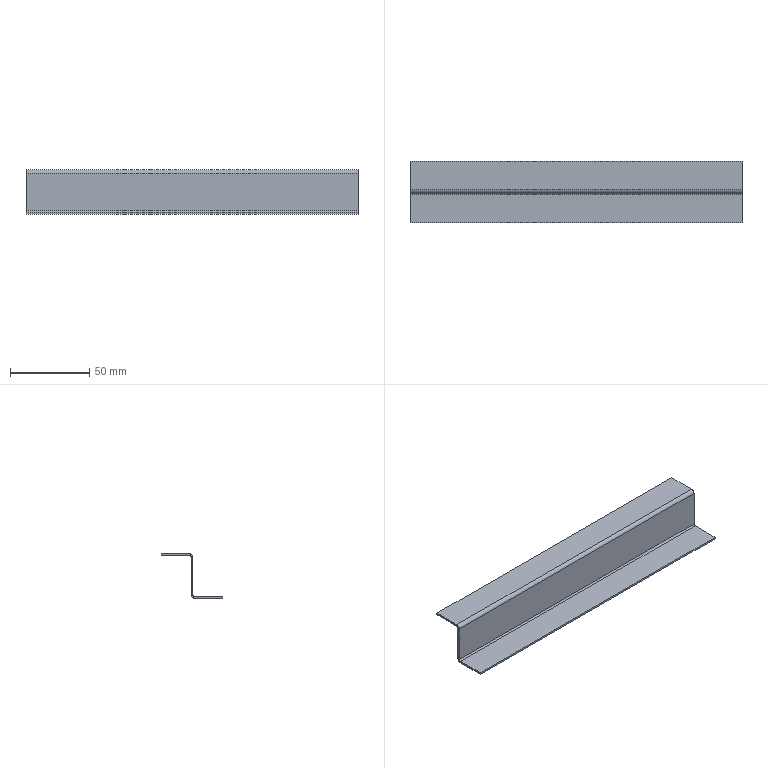Part | SolidWorks | features EdgeFlange 2, FlatPattern 1, HoleWzd 1, SMBaseFlange 1, SheetMetal 1 | 1 solid | 22 faces | box 210 x 38.8 x 28 mm | volume 16185 mm3 | plane 18 | cylinder 4 | commonest cylinder face diameters 2 x2 4.4 x2
STEP:
#1=CARTESIAN_POINT('',(105.,10.,24.6));
#2=VERTEX_POINT('',#1);
#3=CARTESIAN_POINT('',(105.,8.8,24.6));
#4=VERTEX_POINT('',#3);
#5=CARTESIAN_POINT('',(105.,10.,24.6));
#6=DIRECTION('',(0.,-1.,0.));
#7=VECTOR('',#6,1000.);
#8=LINE('',#5,#7);
#9=EDGE_CURVE('',#2,#4,#8,.T.);
#10=ORIENTED_EDGE('',*,*,#9,.T.);
#11=CARTESIAN_POINT('',(105.,8.8,1.));
#12=VERTEX_POINT('',#11);
#13=CARTESIAN_POINT('',(105.,8.8,0.));
#14=DIRECTION('',(0.,0.,-1.));
#15=VECTOR('',#14,1000.);
#16=LINE('',#13,#15);
#17=EDGE_CURVE('',#4,#12,#16,.T.);
#18=ORIENTED_EDGE('',*,*,#17,.T.);
#19=CARTESIAN_POINT('',(105.,10.,1.));
#20=VERTEX_POINT('',#19);
#21=CARTESIAN_POINT('',(105.,10.,1.));
#22=DIRECTION('',(0.,1.,0.));
#23=VECTOR('',#22,1000.);
#24=LINE('',#21,#23);
#25=EDGE_CURVE('',#12,#20,#24,.T.);
#26=ORIENTED_EDGE('',*,*,#25,.T.);
#27=CARTESIAN_POINT('',(105.,10.,0.));
#28=DIRECTION('',(0.,0.,-1.));
#29=VECTOR('',#28,1000.);
#30=LINE('',#27,#29);
#31=EDGE_CURVE('',#2,#20,#30,.T.);
#32=ORIENTED_EDGE('',*,*,#31,.F.);
#33=EDGE_LOOP('',(#10,#18,#26,#32));
#34=FACE_OUTER_BOUND('',#33,.T.);
#35=CARTESIAN_POINT('',(105.,10.,0.));
#36=DIRECTION('',(-1.,0.,0.));
#37=DIRECTION('',(0.,0.,1.));
#38=AXIS2_PLACEMENT_3D('',#35,#36,#37);
#39=PLANE('',#38);
#40=ADVANCED_FACE('',(#34),#39,.F.);
#41=CARTESIAN_POINT('',(-105.,10.,24.6));
#42=VERTEX_POINT('',#41);
#43=CARTESIAN_POINT('',(-105.,8.8,24.6));
#44=VERTEX_POINT('',#43);
#45=CARTESIAN_POINT('',(-105.,10.,24.6));
#46=DIRECTION('',(0.,-1.,0.));
#47=VECTOR('',#46,1000.);
#48=LINE('',#45,#47);
#49=EDGE_CURVE('',#42,#44,#48,.T.);
#50=ORIENTED_EDGE('',*,*,#49,.F.);
#51=CARTESIAN_POINT('',(-105.,10.,1.));
#52=VERTEX_POINT('',#51);
#53=CARTESIAN_POINT('',(-105.,10.,0.));
#54=DIRECTION('',(0.,0.,1.));
#55=VECTOR('',#54,1000.);
#56=LINE('',#53,#55);
#57=EDGE_CURVE('',#52,#42,#56,.T.);
#58=ORIENTED_EDGE('',*,*,#57,.F.);
#59=CARTESIAN_POINT('',(-105.,8.8,1.));
#60=VERTEX_POINT('',#59);
#61=CARTESIAN_POINT('',(-105.,8.8,1.));
#62=DIRECTION('',(0.,1.,0.));
#63=VECTOR('',#62,1000.);
#64=LINE('',#61,#63);
#65=EDGE_CURVE('',#60,#52,#64,.T.);
#66=ORIENTED_EDGE('',*,*,#65,.F.);
#67=CARTESIAN_POINT('',(-105.,8.8,26.8));
#68=DIRECTION('',(0.,0.,1.));
#69=VECTOR('',#68,1000.);
#70=LINE('',#67,#69);
#71=EDGE_CURVE('',#60,#44,#70,.T.);
#72=ORIENTED_EDGE('',*,*,#71,.T.);
#73=EDGE_LOOP('',(#50,#58,#66,#72));
#74=FACE_OUTER_BOUND('',#73,.T.);
#75=CARTESIAN_POINT('',(-105.,10.,26.8));
#76=DIRECTION('',(1.,0.,0.));
#77=DIRECTION('',(0.,0.,-1.));
#78=AXIS2_PLACEMENT_3D('',#75,#76,#77);
#79=PLANE('',#78);
#80=ADVANCED_FACE('',(#74),#79,.F.);
#81=CARTESIAN_POINT('',(105.,10.,24.6));
#82=DIRECTION('',(-1.,0.,0.));
#83=VECTOR('',#82,1000.);
#84=LINE('',#81,#83);
#85=EDGE_CURVE('',#2,#42,#84,.T.);
#86=ORIENTED_EDGE('',*,*,#85,.F.);
#87=ORIENTED_EDGE('',*,*,#31,.T.);
#88=CARTESIAN_POINT('',(105.,10.,1.));
#89=DIRECTION('',(1.,0.,0.));
#90=VECTOR('',#89,1000.);
#91=LINE('',#88,#90);
#92=EDGE_CURVE('',#52,#20,#91,.T.);
#93=ORIENTED_EDGE('',*,*,#92,.F.);
#94=ORIENTED_EDGE('',*,*,#57,.T.);
#95=EDGE_LOOP('',(#86,#87,#93,#94));
#96=FACE_OUTER_BOUND('',#95,.T.);
#97=CARTESIAN_POINT('',(0.,10.,0.));
#98=DIRECTION('',(0.,-1.,0.));
#99=DIRECTION('',(0.,0.,-1.));
#100=AXIS2_PLACEMENT_3D('',#97,#98,#99);
#101=PLANE('',#100);
#102=ADVANCED_FACE('',(#96),#101,.F.);
#103=ORIENTED_EDGE('',*,*,#17,.F.);
#104=CARTESIAN_POINT('',(105.,8.8,24.6));
#105=DIRECTION('',(-1.,0.,0.));
#106=VECTOR('',#105,1000.);
#107=LINE('',#104,#106);
#108=EDGE_CURVE('',#4,#44,#107,.T.);
#109=ORIENTED_EDGE('',*,*,#108,.T.);
#110=ORIENTED_EDGE('',*,*,#71,.F.);
#111=CARTESIAN_POINT('',(105.,8.8,1.));
#112=DIRECTION('',(-1.,0.,0.));
#113=VECTOR('',#112,1000.);
#114=LINE('',#111,#113);
#115=EDGE_CURVE('',#12,#60,#114,.T.);
#116=ORIENTED_EDGE('',*,*,#115,.F.);
#117=EDGE_LOOP('',(#103,#109,#110,#116));
#118=FACE_OUTER_BOUND('',#117,.T.);
#119=CARTESIAN_POINT('',(0.,8.8,0.));
#120=DIRECTION('',(0.,-1.,0.));
#121=DIRECTION('',(0.,0.,-1.));
#122=AXIS2_PLACEMENT_3D('',#119,#120,#121);
#123=PLANE('',#122);
#124=ADVANCED_FACE('',(#118),#123,.T.);
#125=CARTESIAN_POINT('',(-105.,7.8,0.));
#126=VERTEX_POINT('',#125);
#127=CARTESIAN_POINT('',(-105.,-10.,0.));
#128=VERTEX_POINT('',#127);
#129=CARTESIAN_POINT('',(-105.,10.,0.));
#130=DIRECTION('',(0.,-1.,0.));
#131=VECTOR('',#130,1000.);
#132=LINE('',#129,#131);
#133=EDGE_CURVE('',#126,#128,#132,.T.);
#134=ORIENTED_EDGE('',*,*,#133,.F.);
#135=CARTESIAN_POINT('',(-105.,7.8,-1.2));
#136=VERTEX_POINT('',#135);
#137=CARTESIAN_POINT('',(-105.,7.8,0.));
#138=DIRECTION('',(0.,0.,-1.));
#139=VECTOR('',#138,1000.);
#140=LINE('',#137,#139);
#141=EDGE_CURVE('',#126,#136,#140,.T.);
#142=ORIENTED_EDGE('',*,*,#141,.T.);
#143=CARTESIAN_POINT('',(-105.,-10.,-1.2));
#144=VERTEX_POINT('',#143);
#145=CARTESIAN_POINT('',(-105.,10.,-1.2));
#146=DIRECTION('',(0.,-1.,0.));
#147=VECTOR('',#146,1000.);
#148=LINE('',#145,#147);
#149=EDGE_CURVE('',#136,#144,#148,.T.);
#150=ORIENTED_EDGE('',*,*,#149,.T.);
#151=CARTESIAN_POINT('',(-105.,-10.,-1.2));
#152=DIRECTION('',(0.,0.,1.));
#153=VECTOR('',#152,1000.);
#154=LINE('',#151,#153);
#155=EDGE_CURVE('',#144,#128,#154,.T.);
#156=ORIENTED_EDGE('',*,*,#155,.T.);
#157=EDGE_LOOP('',(#134,#142,#150,#156));
#158=FACE_OUTER_BOUND('',#157,.T.);
#159=CARTESIAN_POINT('',(-105.,10.,-1.2));
#160=DIRECTION('',(-1.,0.,0.));
#161=DIRECTION('',(0.,0.,1.));
#162=AXIS2_PLACEMENT_3D('',#159,#160,#161);
#163=PLANE('',#162);
#164=ADVANCED_FACE('',(#158),#163,.T.);
#165=CARTESIAN_POINT('',(105.,7.8,-1.2));
#166=VERTEX_POINT('',#165);
#167=CARTESIAN_POINT('',(-105.,7.8,-1.2));
#168=DIRECTION('',(1.,0.,0.));
#169=VECTOR('',#168,1000.);
#170=LINE('',#167,#169);
#171=EDGE_CURVE('',#136,#166,#170,.T.);
#172=ORIENTED_EDGE('',*,*,#171,.T.);
#173=CARTESIAN_POINT('',(105.,-10.,-1.2));
#174=VERTEX_POINT('',#173);
#175=CARTESIAN_POINT('',(105.,10.,-1.2));
#176=DIRECTION('',(0.,1.,0.));
#177=VECTOR('',#176,1000.);
#178=LINE('',#175,#177);
#179=EDGE_CURVE('',#174,#166,#178,.T.);
#180=ORIENTED_EDGE('',*,*,#179,.F.);
#181=CARTESIAN_POINT('',(-105.,-10.,-1.2));
#182=DIRECTION('',(1.,0.,0.));
#183=VECTOR('',#182,1000.);
#184=LINE('',#181,#183);
#185=EDGE_CURVE('',#144,#174,#184,.T.);
#186=ORIENTED_EDGE('',*,*,#185,.F.);
#187=ORIENTED_EDGE('',*,*,#149,.F.);
#188=EDGE_LOOP('',(#172,#180,#186,#187));
#189=FACE_OUTER_BOUND('',#188,.T.);
#190=CARTESIAN_POINT('',(0.,0.,-1.2));
#191=DIRECTION('',(0.,0.,1.));
#192=DIRECTION('',(1.,0.,0.));
#193=AXIS2_PLACEMENT_3D('',#190,#191,#192);
#194=PLANE('',#193);
#195=ADVANCED_FACE('',(#189),#194,.F.);
#196=CARTESIAN_POINT('',(105.,-10.,0.));
#197=VERTEX_POINT('',#196);
#198=CARTESIAN_POINT('',(105.,7.8,0.));
#199=VERTEX_POINT('',#198);
#200=CARTESIAN_POINT('',(105.,10.,0.));
#201=DIRECTION('',(0.,1.,0.));
#202=VECTOR('',#201,1000.);
#203=LINE('',#200,#202);
#204=EDGE_CURVE('',#197,#199,#203,.T.);
#205=ORIENTED_EDGE('',*,*,#204,.T.);
#206=CARTESIAN_POINT('',(-105.,7.8,0.));
#207=DIRECTION('',(1.,0.,0.));
#208=VECTOR('',#207,1000.);
#209=LINE('',#206,#208);
#210=EDGE_CURVE('',#126,#199,#209,.T.);
#211=ORIENTED_EDGE('',*,*,#210,.F.);
#212=ORIENTED_EDGE('',*,*,#133,.T.);
#213=CARTESIAN_POINT('',(-105.,-10.,0.));
#214=DIRECTION('',(1.,0.,0.));
#215=VECTOR('',#214,1000.);
#216=LINE('',#213,#215);
#217=EDGE_CURVE('',#128,#197,#216,.T.);
#218=ORIENTED_EDGE('',*,*,#217,.T.);
#219=EDGE_LOOP('',(#205,#211,#212,#218));
#220=FACE_OUTER_BOUND('',#219,.T.);
#221=CARTESIAN_POINT('',(0.,0.,0.));
#222=DIRECTION('',(0.,0.,1.));
#223=DIRECTION('',(1.,0.,0.));
#224=AXIS2_PLACEMENT_3D('',#221,#222,#223);
#225=PLANE('',#224);
#226=ADVANCED_FACE('',(#220),#225,.T.);
#227=CARTESIAN_POINT('',(105.,7.8,0.));
#228=DIRECTION('',(0.,0.,-1.));
#229=VECTOR('',#228,1000.);
#230=LINE('',#227,#229);
#231=EDGE_CURVE('',#199,#166,#230,.T.);
#232=ORIENTED_EDGE('',*,*,#231,.F.);
#233=ORIENTED_EDGE('',*,*,#204,.F.);
#234=CARTESIAN_POINT('',(105.,-10.,-1.2));
#235=DIRECTION('',(0.,0.,1.));
#236=VECTOR('',#235,1000.);
#237=LINE('',#234,#236);
#238=EDGE_CURVE('',#174,#197,#237,.T.);
#239=ORIENTED_EDGE('',*,*,#238,.F.);
#240=ORIENTED_EDGE('',*,*,#179,.T.);
#241=EDGE_LOOP('',(#232,#233,#239,#240));
#242=FACE_OUTER_BOUND('',#241,.T.);
#243=CARTESIAN_POINT('',(105.,10.,-1.2));
#244=DIRECTION('',(1.,0.,0.));
#245=DIRECTION('',(0.,0.,-1.));
#246=AXIS2_PLACEMENT_3D('',#243,#244,#245);
#247=PLANE('',#246);
#248=ADVANCED_FACE('',(#242),#247,.T.);
#249=ORIENTED_EDGE('',*,*,#217,.F.);
#250=ORIENTED_EDGE('',*,*,#155,.F.);
#251=ORIENTED_EDGE('',*,*,#185,.T.);
#252=ORIENTED_EDGE('',*,*,#238,.T.);
#253=EDGE_LOOP('',(#249,#250,#251,#252));
#254=FACE_OUTER_BOUND('',#253,.T.);
#255=CARTESIAN_POINT('',(-105.,-10.,-1.2));
#256=DIRECTION('',(0.,-1.,0.));
#257=DIRECTION('',(0.,0.,-1.));
#258=AXIS2_PLACEMENT_3D('',#255,#256,#257);
#259=PLANE('',#258);
#260=ADVANCED_FACE('',(#254),#259,.T.);
#261=ORIENTED_EDGE('',*,*,#25,.F.);
#262=CARTESIAN_POINT('',(105.,7.8,1.));
#263=DIRECTION('',(1.,0.,0.));
#264=DIRECTION('',(0.,0.,1.));
#265=AXIS2_PLACEMENT_3D('',#262,#263,#264);
#266=CIRCLE('',#265,1.);
#267=EDGE_CURVE('',#199,#12,#266,.T.);
#268=ORIENTED_EDGE('',*,*,#267,.F.);
#269=ORIENTED_EDGE('',*,*,#231,.T.);
#270=CARTESIAN_POINT('',(105.,7.8,1.));
#271=DIRECTION('',(1.,0.,0.));
#272=DIRECTION('',(0.,0.,1.));
#273=AXIS2_PLACEMENT_3D('',#270,#271,#272);
#274=CIRCLE('',#273,2.2);
#275=EDGE_CURVE('',#166,#20,#274,.T.);
#276=ORIENTED_EDGE('',*,*,#275,.T.);
#277=EDGE_LOOP('',(#261,#268,#269,#276));
#278=FACE_OUTER_BOUND('',#277,.T.);
#279=CARTESIAN_POINT('',(105.,7.8,1.));
#280=DIRECTION('',(1.,0.,0.));
#281=DIRECTION('',(0.,0.,-1.));
#282=AXIS2_PLACEMENT_3D('',#279,#280,#281);
#283=PLANE('',#282);
#284=ADVANCED_FACE('',(#278),#283,.T.);
#285=CARTESIAN_POINT('',(-105.,7.8,1.));
#286=DIRECTION('',(-1.,0.,0.));
#287=DIRECTION('',(0.,0.,1.));
#288=AXIS2_PLACEMENT_3D('',#285,#286,#287);
#289=CIRCLE('',#288,1.);
#290=EDGE_CURVE('',#60,#126,#289,.T.);
#291=ORIENTED_EDGE('',*,*,#290,.F.);
#292=ORIENTED_EDGE('',*,*,#65,.T.);
#293=CARTESIAN_POINT('',(-105.,7.8,1.));
#294=DIRECTION('',(-1.,0.,0.));
#295=DIRECTION('',(0.,0.,1.));
#296=AXIS2_PLACEMENT_3D('',#293,#294,#295);
#297=CIRCLE('',#296,2.2);
#298=EDGE_CURVE('',#52,#136,#297,.T.);
#299=ORIENTED_EDGE('',*,*,#298,.T.);
#300=ORIENTED_EDGE('',*,*,#141,.F.);
#301=EDGE_LOOP('',(#291,#292,#299,#300));
#302=FACE_OUTER_BOUND('',#301,.T.);
#303=CARTESIAN_POINT('',(-105.,7.8,1.));
#304=DIRECTION('',(1.,0.,0.));
#305=DIRECTION('',(0.,0.,-1.));
#306=AXIS2_PLACEMENT_3D('',#303,#304,#305);
#307=PLANE('',#306);
#308=ADVANCED_FACE('',(#302),#307,.F.);
#309=ORIENTED_EDGE('',*,*,#171,.F.);
#310=ORIENTED_EDGE('',*,*,#298,.F.);
#311=ORIENTED_EDGE('',*,*,#92,.T.);
#312=ORIENTED_EDGE('',*,*,#275,.F.);
#313=EDGE_LOOP('',(#309,#310,#311,#312));
#314=FACE_OUTER_BOUND('',#313,.T.);
#315=CARTESIAN_POINT('',(-105.,7.8,1.));
#316=DIRECTION('',(-1.,0.,0.));
#317=DIRECTION('',(0.,1.,0.));
#318=AXIS2_PLACEMENT_3D('',#315,#316,#317);
#319=CYLINDRICAL_SURFACE('',#318,2.2);
#320=ADVANCED_FACE('',(#314),#319,.T.);
#321=ORIENTED_EDGE('',*,*,#210,.T.);
#322=ORIENTED_EDGE('',*,*,#267,.T.);
#323=ORIENTED_EDGE('',*,*,#115,.T.);
#324=ORIENTED_EDGE('',*,*,#290,.T.);
#325=EDGE_LOOP('',(#321,#322,#323,#324));
#326=FACE_OUTER_BOUND('',#325,.T.);
#327=CARTESIAN_POINT('',(-105.,7.8,1.));
#328=DIRECTION('',(-1.,0.,0.));
#329=DIRECTION('',(0.,1.,0.));
#330=AXIS2_PLACEMENT_3D('',#327,#328,#329);
#331=CYLINDRICAL_SURFACE('',#330,1.);
#332=ADVANCED_FACE('',(#326),#331,.F.);
#333=CARTESIAN_POINT('',(-105.,11.,25.6));
#334=VERTEX_POINT('',#333);
#335=CARTESIAN_POINT('',(-105.,11.,26.8));
#336=VERTEX_POINT('',#335);
#337=CARTESIAN_POINT('',(-105.,11.,26.8));
#338=DIRECTION('',(0.,0.,1.));
#339=VECTOR('',#338,1000.);
#340=LINE('',#337,#339);
#341=EDGE_CURVE('',#334,#336,#340,.T.);
#342=ORIENTED_EDGE('',*,*,#341,.F.);
#343=CARTESIAN_POINT('',(-105.,11.,24.6));
#344=DIRECTION('',(-1.,0.,0.));
#345=DIRECTION('',(0.,0.,-1.));
#346=AXIS2_PLACEMENT_3D('',#343,#344,#345);
#347=CIRCLE('',#346,1.);
#348=EDGE_CURVE('',#42,#334,#347,.T.);
#349=ORIENTED_EDGE('',*,*,#348,.F.);
#350=ORIENTED_EDGE('',*,*,#49,.T.);
#351=CARTESIAN_POINT('',(-105.,11.,24.6));
#352=DIRECTION('',(-1.,0.,0.));
#353=DIRECTION('',(0.,0.,-1.));
#354=AXIS2_PLACEMENT_3D('',#351,#352,#353);
#355=CIRCLE('',#354,2.2);
#356=EDGE_CURVE('',#44,#336,#355,.T.);
#357=ORIENTED_EDGE('',*,*,#356,.T.);
#358=EDGE_LOOP('',(#342,#349,#350,#357));
#359=FACE_OUTER_BOUND('',#358,.T.);
#360=CARTESIAN_POINT('',(-105.,11.,24.6));
#361=DIRECTION('',(-1.,0.,0.));
#362=DIRECTION('',(0.,0.,1.));
#363=AXIS2_PLACEMENT_3D('',#360,#361,#362);
#364=PLANE('',#363);
#365=ADVANCED_FACE('',(#359),#364,.T.);
#366=CARTESIAN_POINT('',(105.,11.,25.6));
#367=VERTEX_POINT('',#366);
#368=CARTESIAN_POINT('',(105.,11.,24.6));
#369=DIRECTION('',(1.,0.,0.));
#370=DIRECTION('',(0.,0.,-1.));
#371=AXIS2_PLACEMENT_3D('',#368,#369,#370);
#372=CIRCLE('',#371,1.);
#373=EDGE_CURVE('',#367,#2,#372,.T.);
#374=ORIENTED_EDGE('',*,*,#373,.F.);
#375=CARTESIAN_POINT('',(105.,11.,26.8));
#376=VERTEX_POINT('',#375);
#377=CARTESIAN_POINT('',(105.,11.,25.6));
#378=DIRECTION('',(0.,0.,1.));
#379=VECTOR('',#378,1000.);
#380=LINE('',#377,#379);
#381=EDGE_CURVE('',#367,#376,#380,.T.);
#382=ORIENTED_EDGE('',*,*,#381,.T.);
#383=CARTESIAN_POINT('',(105.,11.,24.6));
#384=DIRECTION('',(1.,0.,0.));
#385=DIRECTION('',(0.,0.,-1.));
#386=AXIS2_PLACEMENT_3D('',#383,#384,#385);
#387=CIRCLE('',#386,2.2);
#388=EDGE_CURVE('',#376,#4,#387,.T.);
#389=ORIENTED_EDGE('',*,*,#388,.T.);
#390=ORIENTED_EDGE('',*,*,#9,.F.);
#391=EDGE_LOOP('',(#374,#382,#389,#390));
#392=FACE_OUTER_BOUND('',#391,.T.);
#393=CARTESIAN_POINT('',(105.,11.,24.6));
#394=DIRECTION('',(-1.,0.,0.));
#395=DIRECTION('',(0.,0.,1.));
#396=AXIS2_PLACEMENT_3D('',#393,#394,#395);
#397=PLANE('',#396);
#398=ADVANCED_FACE('',(#392),#397,.F.);
#399=ORIENTED_EDGE('',*,*,#108,.F.);
#400=ORIENTED_EDGE('',*,*,#388,.F.);
#401=CARTESIAN_POINT('',(-105.,11.,26.8));
#402=DIRECTION('',(-1.,0.,0.));
#403=VECTOR('',#402,1000.);
#404=LINE('',#401,#403);
#405=EDGE_CURVE('',#376,#336,#404,.T.);
#406=ORIENTED_EDGE('',*,*,#405,.T.);
#407=ORIENTED_EDGE('',*,*,#356,.F.);
#408=EDGE_LOOP('',(#399,#400,#406,#407));
#409=FACE_OUTER_BOUND('',#408,.T.);
#410=CARTESIAN_POINT('',(105.,11.,24.6));
#411=DIRECTION('',(1.,0.,0.));
#412=DIRECTION('',(0.,0.,1.));
#413=AXIS2_PLACEMENT_3D('',#410,#411,#412);
#414=CYLINDRICAL_SURFACE('',#413,2.2);
#415=ADVANCED_FACE('',(#409),#414,.T.);
#416=ORIENTED_EDGE('',*,*,#85,.T.);
#417=ORIENTED_EDGE('',*,*,#348,.T.);
#418=CARTESIAN_POINT('',(-105.,11.,25.6));
#419=DIRECTION('',(1.,0.,0.));
#420=VECTOR('',#419,1000.);
#421=LINE('',#418,#420);
#422=EDGE_CURVE('',#334,#367,#421,.T.);
#423=ORIENTED_EDGE('',*,*,#422,.T.);
#424=ORIENTED_EDGE('',*,*,#373,.T.);
#425=EDGE_LOOP('',(#416,#417,#423,#424));
#426=FACE_OUTER_BOUND('',#425,.T.);
#427=CARTESIAN_POINT('',(105.,11.,24.6));
#428=DIRECTION('',(1.,0.,0.));
#429=DIRECTION('',(0.,0.,1.));
#430=AXIS2_PLACEMENT_3D('',#427,#428,#429);
#431=CYLINDRICAL_SURFACE('',#430,1.);
#432=ADVANCED_FACE('',(#426),#431,.F.);
#433=ORIENTED_EDGE('',*,*,#341,.T.);
#434=CARTESIAN_POINT('',(-105.,28.8,26.8));
#435=VERTEX_POINT('',#434);
#436=CARTESIAN_POINT('',(-105.,0.,26.8));
#437=DIRECTION('',(0.,-1.,0.));
#438=VECTOR('',#437,1000.);
#439=LINE('',#436,#438);
#440=EDGE_CURVE('',#435,#336,#439,.T.);
#441=ORIENTED_EDGE('',*,*,#440,.F.);
#442=CARTESIAN_POINT('',(-105.,28.8,25.6));
#443=VERTEX_POINT('',#442);
#444=CARTESIAN_POINT('',(-105.,28.8,26.8));
#445=DIRECTION('',(0.,0.,-1.));
#446=VECTOR('',#445,1000.);
#447=LINE('',#444,#446);
#448=EDGE_CURVE('',#435,#443,#447,.T.);
#449=ORIENTED_EDGE('',*,*,#448,.T.);
#450=CARTESIAN_POINT('',(-105.,10.,25.6));
#451=DIRECTION('',(0.,-1.,0.));
#452=VECTOR('',#451,1000.);
#453=LINE('',#450,#452);
#454=EDGE_CURVE('',#443,#334,#453,.T.);
#455=ORIENTED_EDGE('',*,*,#454,.T.);
#456=EDGE_LOOP('',(#433,#441,#449,#455));
#457=FACE_OUTER_BOUND('',#456,.T.);
#458=CARTESIAN_POINT('',(-105.,10.,26.8));
#459=DIRECTION('',(1.,0.,0.));
#460=DIRECTION('',(0.,0.,-1.));
#461=AXIS2_PLACEMENT_3D('',#458,#459,#460);
#462=PLANE('',#461);
#463=ADVANCED_FACE('',(#457),#462,.F.);
#464=ORIENTED_EDGE('',*,*,#381,.F.);
#465=CARTESIAN_POINT('',(105.,28.8,25.6));
#466=VERTEX_POINT('',#465);
#467=CARTESIAN_POINT('',(105.,28.8,25.6));
#468=DIRECTION('',(0.,1.,0.));
#469=VECTOR('',#468,1000.);
#470=LINE('',#467,#469);
#471=EDGE_CURVE('',#367,#466,#470,.T.);
#472=ORIENTED_EDGE('',*,*,#471,.T.);
#473=CARTESIAN_POINT('',(105.,28.8,26.8));
#474=VERTEX_POINT('',#473);
#475=CARTESIAN_POINT('',(105.,28.8,26.8));
#476=DIRECTION('',(0.,0.,-1.));
#477=VECTOR('',#476,1000.);
#478=LINE('',#475,#477);
#479=EDGE_CURVE('',#474,#466,#478,.T.);
#480=ORIENTED_EDGE('',*,*,#479,.F.);
#481=CARTESIAN_POINT('',(105.,0.,26.8));
#482=DIRECTION('',(0.,1.,0.));
#483=VECTOR('',#482,1000.);
#484=LINE('',#481,#483);
#485=EDGE_CURVE('',#376,#474,#484,.T.);
#486=ORIENTED_EDGE('',*,*,#485,.F.);
#487=EDGE_LOOP('',(#464,#472,#480,#486));
#488=FACE_OUTER_BOUND('',#487,.T.);
#489=CARTESIAN_POINT('',(105.,28.8,26.8));
#490=DIRECTION('',(-1.,0.,0.));
#491=DIRECTION('',(0.,0.,1.));
#492=AXIS2_PLACEMENT_3D('',#489,#490,#491);
#493=PLANE('',#492);
#494=ADVANCED_FACE('',(#488),#493,.F.);
#495=ORIENTED_EDGE('',*,*,#405,.F.);
#496=ORIENTED_EDGE('',*,*,#485,.T.);
#497=CARTESIAN_POINT('',(0.,28.8,26.8));
#498=DIRECTION('',(-1.,0.,0.));
#499=VECTOR('',#498,1000.);
#500=LINE('',#497,#499);
#501=EDGE_CURVE('',#474,#435,#500,.T.);
#502=ORIENTED_EDGE('',*,*,#501,.T.);
#503=ORIENTED_EDGE('',*,*,#440,.T.);
#504=EDGE_LOOP('',(#495,#496,#502,#503));
#505=FACE_OUTER_BOUND('',#504,.T.);
#506=CARTESIAN_POINT('',(0.,0.,26.8));
#507=DIRECTION('',(0.,0.,-1.));
#508=DIRECTION('',(-1.,0.,0.));
#509=AXIS2_PLACEMENT_3D('',#506,#507,#508);
#510=PLANE('',#509);
#511=ADVANCED_FACE('',(#505),#510,.F.);
#512=ORIENTED_EDGE('',*,*,#471,.F.);
#513=ORIENTED_EDGE('',*,*,#422,.F.);
#514=ORIENTED_EDGE('',*,*,#454,.F.);
#515=CARTESIAN_POINT('',(-105.,28.8,25.6));
#516=DIRECTION('',(-1.,0.,0.));
#517=VECTOR('',#516,1000.);
#518=LINE('',#515,#517);
#519=EDGE_CURVE('',#466,#443,#518,.T.);
#520=ORIENTED_EDGE('',*,*,#519,.F.);
#521=EDGE_LOOP('',(#512,#513,#514,#520));
#522=FACE_OUTER_BOUND('',#521,.T.);
#523=CARTESIAN_POINT('',(0.,0.,25.6));
#524=DIRECTION('',(0.,0.,-1.));
#525=DIRECTION('',(-1.,0.,0.));
#526=AXIS2_PLACEMENT_3D('',#523,#524,#525);
#527=PLANE('',#526);
#528=ADVANCED_FACE('',(#522),#527,.T.);
#529=ORIENTED_EDGE('',*,*,#519,.T.);
#530=ORIENTED_EDGE('',*,*,#448,.F.);
#531=ORIENTED_EDGE('',*,*,#501,.F.);
#532=ORIENTED_EDGE('',*,*,#479,.T.);
#533=EDGE_LOOP('',(#529,#530,#531,#532));
#534=FACE_OUTER_BOUND('',#533,.T.);
#535=CARTESIAN_POINT('',(-105.,28.8,26.8));
#536=DIRECTION('',(0.,-1.,0.));
#537=DIRECTION('',(0.,0.,-1.));
#538=AXIS2_PLACEMENT_3D('',#535,#536,#537);
#539=PLANE('',#538);
#540=ADVANCED_FACE('',(#534),#539,.F.);
#541=CLOSED_SHELL('',(#40,#80,#102,#124,#164,#195,#226,#248,#260,#284,#308,#320,#332,#365,#398,#415,#432,#463,#494,#511,#528,#540));
#542=MANIFOLD_SOLID_BREP('',#541);
#543=CARTESIAN_POINT('',(0.,0.,0.));
#544=DIRECTION('',(0.,0.,1.));
#545=DIRECTION('',(1.,0.,0.));
#546=AXIS2_PLACEMENT_3D('',#543,#544,#545);
#547=(LENGTH_UNIT()NAMED_UNIT(*)SI_UNIT(.MILLI.,.METRE.));
#548=UNCERTAINTY_MEASURE_WITH_UNIT(LENGTH_MEASURE(0.00001),#547,'','');
#549=(NAMED_UNIT(*)PLANE_ANGLE_UNIT()SI_UNIT($,.RADIAN.));
#550=(NAMED_UNIT(*)SI_UNIT($,.STERADIAN.)SOLID_ANGLE_UNIT());
#551=(GEOMETRIC_REPRESENTATION_CONTEXT(3)GLOBAL_UNCERTAINTY_ASSIGNED_CONTEXT((#548))GLOBAL_UNIT_ASSIGNED_CONTEXT((#547,#549,#550))REPRESENTATION_CONTEXT('',''));
#552=ADVANCED_BREP_SHAPE_REPRESENTATION('',(#542,#546),#551);